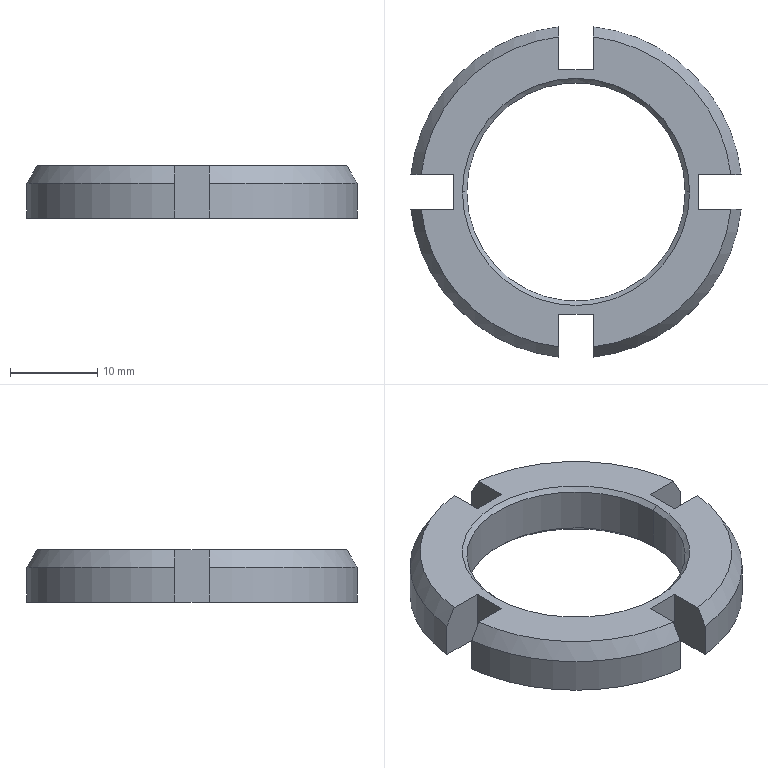Part | SolidWorks | features Chamfer 2, CirPattern 1, Extrusion 1, ICE 1 | 1 solid | 28 faces | box 37.789 x 37.789 x 6 mm | volume 3246 mm3 | plane 14 | cone 8 | cylinder 6 | commonest cylinder face diameters 38 x4 25 x2
STEP:
#1=CARTESIAN_POINT('',(12.5,0.,0.5));
#2=VERTEX_POINT('',#1);
#3=CARTESIAN_POINT('',(-12.5,0.,0.5));
#4=VERTEX_POINT('',#3);
#5=CARTESIAN_POINT('',(0.,0.,0.5));
#6=DIRECTION('',(0.,0.,-1.));
#7=DIRECTION('',(1.,0.,0.));
#8=AXIS2_PLACEMENT_3D('',#5,#6,#7);
#9=CIRCLE('',#8,12.5);
#10=EDGE_CURVE('',#2,#4,#9,.T.);
#11=ORIENTED_EDGE('',*,*,#10,.F.);
#12=CARTESIAN_POINT('',(13.,0.,0.));
#13=VERTEX_POINT('',#12);
#14=CARTESIAN_POINT('',(13.,0.,0.));
#15=DIRECTION('',(0.7071,0.,-0.7071));
#16=VECTOR('',#15,1000.);
#17=LINE('',#14,#16);
#18=EDGE_CURVE('',#2,#13,#17,.T.);
#19=ORIENTED_EDGE('',*,*,#18,.T.);
#20=CARTESIAN_POINT('',(-13.,0.,0.));
#21=VERTEX_POINT('',#20);
#22=CARTESIAN_POINT('',(0.,0.,0.));
#23=DIRECTION('',(0.,0.,1.));
#24=DIRECTION('',(1.,0.,0.));
#25=AXIS2_PLACEMENT_3D('',#22,#23,#24);
#26=CIRCLE('',#25,13.);
#27=EDGE_CURVE('',#21,#13,#26,.T.);
#28=ORIENTED_EDGE('',*,*,#27,.F.);
#29=CARTESIAN_POINT('',(-13.,0.,0.));
#30=DIRECTION('',(-0.7071,0.,-0.7071));
#31=VECTOR('',#30,1000.);
#32=LINE('',#29,#31);
#33=EDGE_CURVE('',#4,#21,#32,.T.);
#34=ORIENTED_EDGE('',*,*,#33,.F.);
#35=EDGE_LOOP('',(#11,#19,#28,#34));
#36=FACE_OUTER_BOUND('',#35,.T.);
#37=CARTESIAN_POINT('',(0.,0.,0.));
#38=DIRECTION('',(0.,0.,-1.));
#39=DIRECTION('',(-1.,0.,0.));
#40=AXIS2_PLACEMENT_3D('',#37,#38,#39);
#41=CONICAL_SURFACE('',#40,13.,0.7854);
#42=ADVANCED_FACE('',(#36),#41,.F.);
#43=CARTESIAN_POINT('',(-12.5,0.,5.5));
#44=VERTEX_POINT('',#43);
#45=CARTESIAN_POINT('',(12.5,0.,5.5));
#46=VERTEX_POINT('',#45);
#47=CARTESIAN_POINT('',(0.,0.,5.5));
#48=DIRECTION('',(0.,0.,1.));
#49=DIRECTION('',(1.,0.,0.));
#50=AXIS2_PLACEMENT_3D('',#47,#48,#49);
#51=CIRCLE('',#50,12.5);
#52=EDGE_CURVE('',#44,#46,#51,.T.);
#53=ORIENTED_EDGE('',*,*,#52,.F.);
#54=CARTESIAN_POINT('',(-13.,0.,6.));
#55=VERTEX_POINT('',#54);
#56=CARTESIAN_POINT('',(-12.5,0.,5.5));
#57=DIRECTION('',(-0.7071,0.,0.7071));
#58=VECTOR('',#57,1000.);
#59=LINE('',#56,#58);
#60=EDGE_CURVE('',#44,#55,#59,.T.);
#61=ORIENTED_EDGE('',*,*,#60,.T.);
#62=CARTESIAN_POINT('',(13.,0.,6.));
#63=VERTEX_POINT('',#62);
#64=CARTESIAN_POINT('',(0.,0.,6.));
#65=DIRECTION('',(0.,0.,-1.));
#66=DIRECTION('',(1.,0.,0.));
#67=AXIS2_PLACEMENT_3D('',#64,#65,#66);
#68=CIRCLE('',#67,13.);
#69=EDGE_CURVE('',#63,#55,#68,.T.);
#70=ORIENTED_EDGE('',*,*,#69,.F.);
#71=CARTESIAN_POINT('',(12.5,0.,5.5));
#72=DIRECTION('',(0.7071,0.,0.7071));
#73=VECTOR('',#72,1000.);
#74=LINE('',#71,#73);
#75=EDGE_CURVE('',#46,#63,#74,.T.);
#76=ORIENTED_EDGE('',*,*,#75,.F.);
#77=EDGE_LOOP('',(#53,#61,#70,#76));
#78=FACE_OUTER_BOUND('',#77,.T.);
#79=CARTESIAN_POINT('',(0.,0.,5.5));
#80=DIRECTION('',(0.,0.,1.));
#81=DIRECTION('',(1.,0.,0.));
#82=AXIS2_PLACEMENT_3D('',#79,#80,#81);
#83=CONICAL_SURFACE('',#82,12.5,0.7854);
#84=ADVANCED_FACE('',(#78),#83,.F.);
#85=ORIENTED_EDGE('',*,*,#52,.T.);
#86=CARTESIAN_POINT('',(12.5,0.,6.));
#87=DIRECTION('',(0.,0.,-1.));
#88=VECTOR('',#87,1000.);
#89=LINE('',#86,#88);
#90=EDGE_CURVE('',#46,#2,#89,.T.);
#91=ORIENTED_EDGE('',*,*,#90,.T.);
#92=ORIENTED_EDGE('',*,*,#10,.T.);
#93=CARTESIAN_POINT('',(-12.5,0.,6.));
#94=DIRECTION('',(0.,0.,-1.));
#95=VECTOR('',#94,1000.);
#96=LINE('',#93,#95);
#97=EDGE_CURVE('',#44,#4,#96,.T.);
#98=ORIENTED_EDGE('',*,*,#97,.F.);
#99=EDGE_LOOP('',(#85,#91,#92,#98));
#100=FACE_OUTER_BOUND('',#99,.T.);
#101=CARTESIAN_POINT('',(0.,0.,6.));
#102=DIRECTION('',(0.,0.,-1.));
#103=DIRECTION('',(-1.,0.,0.));
#104=AXIS2_PLACEMENT_3D('',#101,#102,#103);
#105=CYLINDRICAL_SURFACE('',#104,12.5);
#106=ADVANCED_FACE('',(#100),#105,.F.);
#107=ORIENTED_EDGE('',*,*,#69,.T.);
#108=CARTESIAN_POINT('',(0.,0.,6.));
#109=DIRECTION('',(0.,0.,-1.));
#110=DIRECTION('',(1.,0.,0.));
#111=AXIS2_PLACEMENT_3D('',#108,#109,#110);
#112=CIRCLE('',#111,13.);
#113=EDGE_CURVE('',#55,#63,#112,.T.);
#114=ORIENTED_EDGE('',*,*,#113,.T.);
#115=EDGE_LOOP('',(#107,#114));
#116=FACE_BOUND('',#115,.T.);
#117=CARTESIAN_POINT('',(2.,-17.733,6.));
#118=VERTEX_POINT('',#117);
#119=CARTESIAN_POINT('',(2.,-14.,6.));
#120=VERTEX_POINT('',#119);
#121=CARTESIAN_POINT('',(2.,-20.,6.));
#122=DIRECTION('',(0.,1.,0.));
#123=VECTOR('',#122,1000.);
#124=LINE('',#121,#123);
#125=EDGE_CURVE('',#118,#120,#124,.T.);
#126=ORIENTED_EDGE('',*,*,#125,.F.);
#127=CARTESIAN_POINT('',(17.733,-2.,6.));
#128=VERTEX_POINT('',#127);
#129=CARTESIAN_POINT('',(0.,0.,6.));
#130=DIRECTION('',(0.,0.,1.));
#131=DIRECTION('',(1.,0.,0.));
#132=AXIS2_PLACEMENT_3D('',#129,#130,#131);
#133=CIRCLE('',#132,17.845);
#134=EDGE_CURVE('',#118,#128,#133,.T.);
#135=ORIENTED_EDGE('',*,*,#134,.T.);
#136=CARTESIAN_POINT('',(14.,-2.,6.));
#137=VERTEX_POINT('',#136);
#138=CARTESIAN_POINT('',(20.,-2.,6.));
#139=DIRECTION('',(-1.,0.,0.));
#140=VECTOR('',#139,1000.);
#141=LINE('',#138,#140);
#142=EDGE_CURVE('',#128,#137,#141,.T.);
#143=ORIENTED_EDGE('',*,*,#142,.T.);
#144=CARTESIAN_POINT('',(14.,2.,6.));
#145=VERTEX_POINT('',#144);
#146=CARTESIAN_POINT('',(14.,-2.,6.));
#147=DIRECTION('',(0.,-1.,0.));
#148=VECTOR('',#147,1000.);
#149=LINE('',#146,#148);
#150=EDGE_CURVE('',#145,#137,#149,.T.);
#151=ORIENTED_EDGE('',*,*,#150,.F.);
#152=CARTESIAN_POINT('',(17.733,2.,6.));
#153=VERTEX_POINT('',#152);
#154=CARTESIAN_POINT('',(20.,2.,6.));
#155=DIRECTION('',(-1.,0.,0.));
#156=VECTOR('',#155,1000.);
#157=LINE('',#154,#156);
#158=EDGE_CURVE('',#153,#145,#157,.T.);
#159=ORIENTED_EDGE('',*,*,#158,.F.);
#160=CARTESIAN_POINT('',(2.,17.733,6.));
#161=VERTEX_POINT('',#160);
#162=CARTESIAN_POINT('',(0.,0.,6.));
#163=DIRECTION('',(0.,0.,1.));
#164=DIRECTION('',(1.,0.,0.));
#165=AXIS2_PLACEMENT_3D('',#162,#163,#164);
#166=CIRCLE('',#165,17.845);
#167=EDGE_CURVE('',#153,#161,#166,.T.);
#168=ORIENTED_EDGE('',*,*,#167,.T.);
#169=CARTESIAN_POINT('',(2.,14.,6.));
#170=VERTEX_POINT('',#169);
#171=CARTESIAN_POINT('',(2.,20.,6.));
#172=DIRECTION('',(0.,-1.,0.));
#173=VECTOR('',#172,1000.);
#174=LINE('',#171,#173);
#175=EDGE_CURVE('',#161,#170,#174,.T.);
#176=ORIENTED_EDGE('',*,*,#175,.T.);
#177=CARTESIAN_POINT('',(-2.,14.,6.));
#178=VERTEX_POINT('',#177);
#179=CARTESIAN_POINT('',(2.,14.,6.));
#180=DIRECTION('',(1.,0.,0.));
#181=VECTOR('',#180,1000.);
#182=LINE('',#179,#181);
#183=EDGE_CURVE('',#178,#170,#182,.T.);
#184=ORIENTED_EDGE('',*,*,#183,.F.);
#185=CARTESIAN_POINT('',(-2.,17.733,6.));
#186=VERTEX_POINT('',#185);
#187=CARTESIAN_POINT('',(-2.,20.,6.));
#188=DIRECTION('',(0.,-1.,0.));
#189=VECTOR('',#188,1000.);
#190=LINE('',#187,#189);
#191=EDGE_CURVE('',#186,#178,#190,.T.);
#192=ORIENTED_EDGE('',*,*,#191,.F.);
#193=CARTESIAN_POINT('',(-17.733,2.,6.));
#194=VERTEX_POINT('',#193);
#195=CARTESIAN_POINT('',(0.,0.,6.));
#196=DIRECTION('',(0.,0.,1.));
#197=DIRECTION('',(1.,0.,0.));
#198=AXIS2_PLACEMENT_3D('',#195,#196,#197);
#199=CIRCLE('',#198,17.845);
#200=EDGE_CURVE('',#186,#194,#199,.T.);
#201=ORIENTED_EDGE('',*,*,#200,.T.);
#202=CARTESIAN_POINT('',(-14.,2.,6.));
#203=VERTEX_POINT('',#202);
#204=CARTESIAN_POINT('',(-20.,2.,6.));
#205=DIRECTION('',(1.,0.,0.));
#206=VECTOR('',#205,1000.);
#207=LINE('',#204,#206);
#208=EDGE_CURVE('',#194,#203,#207,.T.);
#209=ORIENTED_EDGE('',*,*,#208,.T.);
#210=CARTESIAN_POINT('',(-14.,-2.,6.));
#211=VERTEX_POINT('',#210);
#212=CARTESIAN_POINT('',(-14.,2.,6.));
#213=DIRECTION('',(0.,1.,0.));
#214=VECTOR('',#213,1000.);
#215=LINE('',#212,#214);
#216=EDGE_CURVE('',#211,#203,#215,.T.);
#217=ORIENTED_EDGE('',*,*,#216,.F.);
#218=CARTESIAN_POINT('',(-17.733,-2.,6.));
#219=VERTEX_POINT('',#218);
#220=CARTESIAN_POINT('',(-20.,-2.,6.));
#221=DIRECTION('',(1.,0.,0.));
#222=VECTOR('',#221,1000.);
#223=LINE('',#220,#222);
#224=EDGE_CURVE('',#219,#211,#223,.T.);
#225=ORIENTED_EDGE('',*,*,#224,.F.);
#226=CARTESIAN_POINT('',(-2.,-17.733,6.));
#227=VERTEX_POINT('',#226);
#228=CARTESIAN_POINT('',(0.,0.,6.));
#229=DIRECTION('',(0.,0.,1.));
#230=DIRECTION('',(1.,0.,0.));
#231=AXIS2_PLACEMENT_3D('',#228,#229,#230);
#232=CIRCLE('',#231,17.845);
#233=EDGE_CURVE('',#219,#227,#232,.T.);
#234=ORIENTED_EDGE('',*,*,#233,.T.);
#235=CARTESIAN_POINT('',(-2.,-14.,6.));
#236=VERTEX_POINT('',#235);
#237=CARTESIAN_POINT('',(-2.,-20.,6.));
#238=DIRECTION('',(0.,1.,0.));
#239=VECTOR('',#238,1000.);
#240=LINE('',#237,#239);
#241=EDGE_CURVE('',#227,#236,#240,.T.);
#242=ORIENTED_EDGE('',*,*,#241,.T.);
#243=CARTESIAN_POINT('',(-2.,-14.,6.));
#244=DIRECTION('',(-1.,0.,0.));
#245=VECTOR('',#244,1000.);
#246=LINE('',#243,#245);
#247=EDGE_CURVE('',#120,#236,#246,.T.);
#248=ORIENTED_EDGE('',*,*,#247,.F.);
#249=EDGE_LOOP('',(#126,#135,#143,#151,#159,#168,#176,#184,#192,#201,#209,#217,#225,#234,#242,#248));
#250=FACE_OUTER_BOUND('',#249,.T.);
#251=CARTESIAN_POINT('',(0.,0.,6.));
#252=DIRECTION('',(0.,0.,1.));
#253=DIRECTION('',(1.,0.,0.));
#254=AXIS2_PLACEMENT_3D('',#251,#252,#253);
#255=PLANE('',#254);
#256=ADVANCED_FACE('',(#116,#250),#255,.T.);
#257=ORIENTED_EDGE('',*,*,#27,.T.);
#258=CARTESIAN_POINT('',(0.,0.,0.));
#259=DIRECTION('',(0.,0.,1.));
#260=DIRECTION('',(1.,0.,0.));
#261=AXIS2_PLACEMENT_3D('',#258,#259,#260);
#262=CIRCLE('',#261,13.);
#263=EDGE_CURVE('',#13,#21,#262,.T.);
#264=ORIENTED_EDGE('',*,*,#263,.T.);
#265=EDGE_LOOP('',(#257,#264));
#266=FACE_BOUND('',#265,.T.);
#267=CARTESIAN_POINT('',(-2.,18.894,0.));
#268=VERTEX_POINT('',#267);
#269=CARTESIAN_POINT('',(-2.,14.,0.));
#270=VERTEX_POINT('',#269);
#271=CARTESIAN_POINT('',(-2.,20.,0.));
#272=DIRECTION('',(0.,-1.,0.));
#273=VECTOR('',#272,1000.);
#274=LINE('',#271,#273);
#275=EDGE_CURVE('',#268,#270,#274,.T.);
#276=ORIENTED_EDGE('',*,*,#275,.T.);
#277=CARTESIAN_POINT('',(2.,14.,0.));
#278=VERTEX_POINT('',#277);
#279=CARTESIAN_POINT('',(2.,14.,0.));
#280=DIRECTION('',(-1.,0.,0.));
#281=VECTOR('',#280,1000.);
#282=LINE('',#279,#281);
#283=EDGE_CURVE('',#278,#270,#282,.T.);
#284=ORIENTED_EDGE('',*,*,#283,.F.);
#285=CARTESIAN_POINT('',(2.,18.894,0.));
#286=VERTEX_POINT('',#285);
#287=CARTESIAN_POINT('',(2.,20.,0.));
#288=DIRECTION('',(0.,-1.,0.));
#289=VECTOR('',#288,1000.);
#290=LINE('',#287,#289);
#291=EDGE_CURVE('',#286,#278,#290,.T.);
#292=ORIENTED_EDGE('',*,*,#291,.F.);
#293=CARTESIAN_POINT('',(18.894,2.,0.));
#294=VERTEX_POINT('',#293);
#295=CARTESIAN_POINT('',(0.,0.,0.));
#296=DIRECTION('',(0.,0.,1.));
#297=DIRECTION('',(1.,0.,0.));
#298=AXIS2_PLACEMENT_3D('',#295,#296,#297);
#299=CIRCLE('',#298,19.);
#300=EDGE_CURVE('',#294,#286,#299,.T.);
#301=ORIENTED_EDGE('',*,*,#300,.F.);
#302=CARTESIAN_POINT('',(14.,2.,0.));
#303=VERTEX_POINT('',#302);
#304=CARTESIAN_POINT('',(20.,2.,0.));
#305=DIRECTION('',(-1.,0.,0.));
#306=VECTOR('',#305,1000.);
#307=LINE('',#304,#306);
#308=EDGE_CURVE('',#294,#303,#307,.T.);
#309=ORIENTED_EDGE('',*,*,#308,.T.);
#310=CARTESIAN_POINT('',(14.,-2.,0.));
#311=VERTEX_POINT('',#310);
#312=CARTESIAN_POINT('',(14.,-2.,0.));
#313=DIRECTION('',(0.,1.,0.));
#314=VECTOR('',#313,1000.);
#315=LINE('',#312,#314);
#316=EDGE_CURVE('',#311,#303,#315,.T.);
#317=ORIENTED_EDGE('',*,*,#316,.F.);
#318=CARTESIAN_POINT('',(18.894,-2.,0.));
#319=VERTEX_POINT('',#318);
#320=CARTESIAN_POINT('',(20.,-2.,0.));
#321=DIRECTION('',(-1.,0.,0.));
#322=VECTOR('',#321,1000.);
#323=LINE('',#320,#322);
#324=EDGE_CURVE('',#319,#311,#323,.T.);
#325=ORIENTED_EDGE('',*,*,#324,.F.);
#326=CARTESIAN_POINT('',(2.,-18.894,0.));
#327=VERTEX_POINT('',#326);
#328=CARTESIAN_POINT('',(0.,0.,0.));
#329=DIRECTION('',(0.,0.,1.));
#330=DIRECTION('',(1.,0.,0.));
#331=AXIS2_PLACEMENT_3D('',#328,#329,#330);
#332=CIRCLE('',#331,19.);
#333=EDGE_CURVE('',#327,#319,#332,.T.);
#334=ORIENTED_EDGE('',*,*,#333,.F.);
#335=CARTESIAN_POINT('',(2.,-14.,0.));
#336=VERTEX_POINT('',#335);
#337=CARTESIAN_POINT('',(2.,-20.,0.));
#338=DIRECTION('',(0.,1.,0.));
#339=VECTOR('',#338,1000.);
#340=LINE('',#337,#339);
#341=EDGE_CURVE('',#327,#336,#340,.T.);
#342=ORIENTED_EDGE('',*,*,#341,.T.);
#343=CARTESIAN_POINT('',(-2.,-14.,0.));
#344=VERTEX_POINT('',#343);
#345=CARTESIAN_POINT('',(-2.,-14.,0.));
#346=DIRECTION('',(1.,0.,0.));
#347=VECTOR('',#346,1000.);
#348=LINE('',#345,#347);
#349=EDGE_CURVE('',#344,#336,#348,.T.);
#350=ORIENTED_EDGE('',*,*,#349,.F.);
#351=CARTESIAN_POINT('',(-2.,-18.894,0.));
#352=VERTEX_POINT('',#351);
#353=CARTESIAN_POINT('',(-2.,-20.,0.));
#354=DIRECTION('',(0.,1.,0.));
#355=VECTOR('',#354,1000.);
#356=LINE('',#353,#355);
#357=EDGE_CURVE('',#352,#344,#356,.T.);
#358=ORIENTED_EDGE('',*,*,#357,.F.);
#359=CARTESIAN_POINT('',(-18.894,-2.,0.));
#360=VERTEX_POINT('',#359);
#361=CARTESIAN_POINT('',(0.,0.,0.));
#362=DIRECTION('',(0.,0.,1.));
#363=DIRECTION('',(1.,0.,0.));
#364=AXIS2_PLACEMENT_3D('',#361,#362,#363);
#365=CIRCLE('',#364,19.);
#366=EDGE_CURVE('',#360,#352,#365,.T.);
#367=ORIENTED_EDGE('',*,*,#366,.F.);
#368=CARTESIAN_POINT('',(-14.,-2.,0.));
#369=VERTEX_POINT('',#368);
#370=CARTESIAN_POINT('',(-20.,-2.,0.));
#371=DIRECTION('',(1.,0.,0.));
#372=VECTOR('',#371,1000.);
#373=LINE('',#370,#372);
#374=EDGE_CURVE('',#360,#369,#373,.T.);
#375=ORIENTED_EDGE('',*,*,#374,.T.);
#376=CARTESIAN_POINT('',(-14.,2.,0.));
#377=VERTEX_POINT('',#376);
#378=CARTESIAN_POINT('',(-14.,2.,0.));
#379=DIRECTION('',(0.,-1.,0.));
#380=VECTOR('',#379,1000.);
#381=LINE('',#378,#380);
#382=EDGE_CURVE('',#377,#369,#381,.T.);
#383=ORIENTED_EDGE('',*,*,#382,.F.);
#384=CARTESIAN_POINT('',(-18.894,2.,0.));
#385=VERTEX_POINT('',#384);
#386=CARTESIAN_POINT('',(-20.,2.,0.));
#387=DIRECTION('',(1.,0.,0.));
#388=VECTOR('',#387,1000.);
#389=LINE('',#386,#388);
#390=EDGE_CURVE('',#385,#377,#389,.T.);
#391=ORIENTED_EDGE('',*,*,#390,.F.);
#392=CARTESIAN_POINT('',(0.,0.,0.));
#393=DIRECTION('',(0.,0.,1.));
#394=DIRECTION('',(1.,0.,0.));
#395=AXIS2_PLACEMENT_3D('',#392,#393,#394);
#396=CIRCLE('',#395,19.);
#397=EDGE_CURVE('',#268,#385,#396,.T.);
#398=ORIENTED_EDGE('',*,*,#397,.F.);
#399=EDGE_LOOP('',(#276,#284,#292,#301,#309,#317,#325,#334,#342,#350,#358,#367,#375,#383,#391,#398));
#400=FACE_OUTER_BOUND('',#399,.T.);
#401=CARTESIAN_POINT('',(0.,0.,0.));
#402=DIRECTION('',(0.,0.,1.));
#403=DIRECTION('',(1.,0.,0.));
#404=AXIS2_PLACEMENT_3D('',#401,#402,#403);
#405=PLANE('',#404);
#406=ADVANCED_FACE('',(#266,#400),#405,.F.);
#407=CARTESIAN_POINT('',(-18.894,2.,4.));
#408=VERTEX_POINT('',#407);
#409=CARTESIAN_POINT('',(-18.894,2.,6.));
#410=DIRECTION('',(0.,0.,-1.));
#411=VECTOR('',#410,1000.);
#412=LINE('',#409,#411);
#413=EDGE_CURVE('',#408,#385,#412,.T.);
#414=ORIENTED_EDGE('',*,*,#413,.F.);
#415=CARTESIAN_POINT('',(-2.,18.894,4.));
#416=VERTEX_POINT('',#415);
#417=CARTESIAN_POINT('',(0.,0.,4.));
#418=DIRECTION('',(0.,0.,-1.));
#419=DIRECTION('',(1.,0.,0.));
#420=AXIS2_PLACEMENT_3D('',#417,#418,#419);
#421=CIRCLE('',#420,19.);
#422=EDGE_CURVE('',#408,#416,#421,.T.);
#423=ORIENTED_EDGE('',*,*,#422,.T.);
#424=CARTESIAN_POINT('',(-2.,18.894,6.));
#425=DIRECTION('',(0.,0.,1.));
#426=VECTOR('',#425,1000.);
#427=LINE('',#424,#426);
#428=EDGE_CURVE('',#268,#416,#427,.T.);
#429=ORIENTED_EDGE('',*,*,#428,.F.);
#430=ORIENTED_EDGE('',*,*,#397,.T.);
#431=EDGE_LOOP('',(#414,#423,#429,#430));
#432=FACE_OUTER_BOUND('',#431,.T.);
#433=CARTESIAN_POINT('',(0.,0.,6.));
#434=DIRECTION('',(0.,0.,-1.));
#435=DIRECTION('',(-1.,0.,0.));
#436=AXIS2_PLACEMENT_3D('',#433,#434,#435);
#437=CYLINDRICAL_SURFACE('',#436,19.);
#438=ADVANCED_FACE('',(#432),#437,.T.);
#439=CARTESIAN_POINT('',(2.,18.894,4.));
#440=VERTEX_POINT('',#439);
#441=CARTESIAN_POINT('',(2.,18.894,6.));
#442=DIRECTION('',(0.,0.,-1.));
#443=VECTOR('',#442,1000.);
#444=LINE('',#441,#443);
#445=EDGE_CURVE('',#440,#286,#444,.T.);
#446=ORIENTED_EDGE('',*,*,#445,.F.);
#447=CARTESIAN_POINT('',(18.894,2.,4.));
#448=VERTEX_POINT('',#447);
#449=CARTESIAN_POINT('',(0.,0.,4.));
#450=DIRECTION('',(0.,0.,-1.));
#451=DIRECTION('',(1.,0.,0.));
#452=AXIS2_PLACEMENT_3D('',#449,#450,#451);
#453=CIRCLE('',#452,19.);
#454=EDGE_CURVE('',#440,#448,#453,.T.);
#455=ORIENTED_EDGE('',*,*,#454,.T.);
#456=CARTESIAN_POINT('',(18.894,2.,6.));
#457=DIRECTION('',(0.,0.,1.));
#458=VECTOR('',#457,1000.);
#459=LINE('',#456,#458);
#460=EDGE_CURVE('',#294,#448,#459,.T.);
#461=ORIENTED_EDGE('',*,*,#460,.F.);
#462=ORIENTED_EDGE('',*,*,#300,.T.);
#463=EDGE_LOOP('',(#446,#455,#461,#462));
#464=FACE_OUTER_BOUND('',#463,.T.);
#465=CARTESIAN_POINT('',(0.,0.,6.));
#466=DIRECTION('',(0.,0.,-1.));
#467=DIRECTION('',(-1.,0.,0.));
#468=AXIS2_PLACEMENT_3D('',#465,#466,#467);
#469=CYLINDRICAL_SURFACE('',#468,19.);
#470=ADVANCED_FACE('',(#464),#469,.T.);
#471=CARTESIAN_POINT('',(-2.,-18.894,4.));
#472=VERTEX_POINT('',#471);
#473=CARTESIAN_POINT('',(-2.,-18.894,6.));
#474=DIRECTION('',(0.,0.,-1.));
#475=VECTOR('',#474,1000.);
#476=LINE('',#473,#475);
#477=EDGE_CURVE('',#472,#352,#476,.T.);
#478=ORIENTED_EDGE('',*,*,#477,.F.);
#479=CARTESIAN_POINT('',(-18.894,-2.,4.));
#480=VERTEX_POINT('',#479);
#481=CARTESIAN_POINT('',(0.,0.,4.));
#482=DIRECTION('',(0.,0.,-1.));
#483=DIRECTION('',(1.,0.,0.));
#484=AXIS2_PLACEMENT_3D('',#481,#482,#483);
#485=CIRCLE('',#484,19.);
#486=EDGE_CURVE('',#472,#480,#485,.T.);
#487=ORIENTED_EDGE('',*,*,#486,.T.);
#488=CARTESIAN_POINT('',(-18.894,-2.,6.));
#489=DIRECTION('',(0.,0.,1.));
#490=VECTOR('',#489,1000.);
#491=LINE('',#488,#490);
#492=EDGE_CURVE('',#360,#480,#491,.T.);
#493=ORIENTED_EDGE('',*,*,#492,.F.);
#494=ORIENTED_EDGE('',*,*,#366,.T.);
#495=EDGE_LOOP('',(#478,#487,#493,#494));
#496=FACE_OUTER_BOUND('',#495,.T.);
#497=CARTESIAN_POINT('',(0.,0.,6.));
#498=DIRECTION('',(0.,0.,-1.));
#499=DIRECTION('',(-1.,0.,0.));
#500=AXIS2_PLACEMENT_3D('',#497,#498,#499);
#501=CYLINDRICAL_SURFACE('',#500,19.);
#502=ADVANCED_FACE('',(#496),#501,.T.);
#503=CARTESIAN_POINT('',(18.894,-2.,4.));
#504=VERTEX_POINT('',#503);
#505=CARTESIAN_POINT('',(18.894,-2.,6.));
#506=DIRECTION('',(0.,0.,-1.));
#507=VECTOR('',#506,1000.);
#508=LINE('',#505,#507);
#509=EDGE_CURVE('',#504,#319,#508,.T.);
#510=ORIENTED_EDGE('',*,*,#509,.F.);
#511=CARTESIAN_POINT('',(2.,-18.894,4.));
#512=VERTEX_POINT('',#511);
#513=CARTESIAN_POINT('',(0.,0.,4.));
#514=DIRECTION('',(0.,0.,-1.));
#515=DIRECTION('',(1.,0.,0.));
#516=AXIS2_PLACEMENT_3D('',#513,#514,#515);
#517=CIRCLE('',#516,19.);
#518=EDGE_CURVE('',#504,#512,#517,.T.);
#519=ORIENTED_EDGE('',*,*,#518,.T.);
#520=CARTESIAN_POINT('',(2.,-18.894,6.));
#521=DIRECTION('',(0.,0.,1.));
#522=VECTOR('',#521,1000.);
#523=LINE('',#520,#522);
#524=EDGE_CURVE('',#327,#512,#523,.T.);
#525=ORIENTED_EDGE('',*,*,#524,.F.);
#526=ORIENTED_EDGE('',*,*,#333,.T.);
#527=EDGE_LOOP('',(#510,#519,#525,#526));
#528=FACE_OUTER_BOUND('',#527,.T.);
#529=CARTESIAN_POINT('',(0.,0.,6.));
#530=DIRECTION('',(0.,0.,-1.));
#531=DIRECTION('',(-1.,0.,0.));
#532=AXIS2_PLACEMENT_3D('',#529,#530,#531);
#533=CYLINDRICAL_SURFACE('',#532,19.);
#534=ADVANCED_FACE('',(#528),#533,.T.);
#535=ORIENTED_EDGE('',*,*,#90,.F.);
#536=CARTESIAN_POINT('',(0.,0.,5.5));
#537=DIRECTION('',(0.,0.,1.));
#538=DIRECTION('',(1.,0.,0.));
#539=AXIS2_PLACEMENT_3D('',#536,#537,#538);
#540=CIRCLE('',#539,12.5);
#541=EDGE_CURVE('',#46,#44,#540,.T.);
#542=ORIENTED_EDGE('',*,*,#541,.T.);
#543=ORIENTED_EDGE('',*,*,#97,.T.);
#544=CARTESIAN_POINT('',(0.,0.,0.5));
#545=DIRECTION('',(0.,0.,-1.));
#546=DIRECTION('',(1.,0.,0.));
#547=AXIS2_PLACEMENT_3D('',#544,#545,#546);
#548=CIRCLE('',#547,12.5);
#549=EDGE_CURVE('',#4,#2,#548,.T.);
#550=ORIENTED_EDGE('',*,*,#549,.T.);
#551=EDGE_LOOP('',(#535,#542,#543,#550));
#552=FACE_OUTER_BOUND('',#551,.T.);
#553=CARTESIAN_POINT('',(0.,0.,6.));
#554=DIRECTION('',(0.,0.,-1.));
#555=DIRECTION('',(-1.,0.,0.));
#556=AXIS2_PLACEMENT_3D('',#553,#554,#555);
#557=CYLINDRICAL_SURFACE('',#556,12.5);
#558=ADVANCED_FACE('',(#552),#557,.F.);
#559=ORIENTED_EDGE('',*,*,#460,.T.);
#560=CARTESIAN_POINT('',(18.894,2.,4.));
#561=CARTESIAN_POINT('',(18.507,2.,4.667));
#562=CARTESIAN_POINT('',(18.12,2.,5.333));
#563=CARTESIAN_POINT('',(17.733,2.,6.));
#564=B_SPLINE_CURVE_WITH_KNOTS('',3,(#560,#561,#562,#563),.UNSPECIFIED.,.F.,.F.,(4,4),(0.,0.002313),.UNSPECIFIED.);
#565=EDGE_CURVE('',#448,#153,#564,.T.);
#566=ORIENTED_EDGE('',*,*,#565,.T.);
#567=ORIENTED_EDGE('',*,*,#158,.T.);
#568=CARTESIAN_POINT('',(14.,2.,0.));
#569=DIRECTION('',(0.,0.,1.));
#570=VECTOR('',#569,1000.);
#571=LINE('',#568,#570);
#572=EDGE_CURVE('',#303,#145,#571,.T.);
#573=ORIENTED_EDGE('',*,*,#572,.F.);
#574=ORIENTED_EDGE('',*,*,#308,.F.);
#575=EDGE_LOOP('',(#559,#566,#567,#573,#574));
#576=FACE_OUTER_BOUND('',#575,.T.);
#577=CARTESIAN_POINT('',(20.,2.,0.));
#578=DIRECTION('',(0.,-1.,0.));
#579=DIRECTION('',(0.,0.,-1.));
#580=AXIS2_PLACEMENT_3D('',#577,#578,#579);
#581=PLANE('',#580);
#582=ADVANCED_FACE('',(#576),#581,.T.);
#583=ORIENTED_EDGE('',*,*,#142,.F.);
#584=CARTESIAN_POINT('',(17.733,-2.,6.));
#585=CARTESIAN_POINT('',(18.12,-2.,5.333));
#586=CARTESIAN_POINT('',(18.507,-2.,4.667));
#587=CARTESIAN_POINT('',(18.894,-2.,4.));
#588=B_SPLINE_CURVE_WITH_KNOTS('',3,(#584,#585,#586,#587),.UNSPECIFIED.,.F.,.F.,(4,4),(0.,0.002313),.UNSPECIFIED.);
#589=EDGE_CURVE('',#128,#504,#588,.T.);
#590=ORIENTED_EDGE('',*,*,#589,.T.);
#591=ORIENTED_EDGE('',*,*,#509,.T.);
#592=ORIENTED_EDGE('',*,*,#324,.T.);
#593=CARTESIAN_POINT('',(14.,-2.,0.));
#594=DIRECTION('',(0.,0.,-1.));
#595=VECTOR('',#594,1000.);
#596=LINE('',#593,#595);
#597=EDGE_CURVE('',#137,#311,#596,.T.);
#598=ORIENTED_EDGE('',*,*,#597,.F.);
#599=EDGE_LOOP('',(#583,#590,#591,#592,#598));
#600=FACE_OUTER_BOUND('',#599,.T.);
#601=CARTESIAN_POINT('',(20.,-2.,0.));
#602=DIRECTION('',(0.,1.,0.));
#603=DIRECTION('',(0.,0.,1.));
#604=AXIS2_PLACEMENT_3D('',#601,#602,#603);
#605=PLANE('',#604);
#606=ADVANCED_FACE('',(#600),#605,.T.);
#607=ORIENTED_EDGE('',*,*,#316,.T.);
#608=ORIENTED_EDGE('',*,*,#572,.T.);
#609=ORIENTED_EDGE('',*,*,#150,.T.);
#610=ORIENTED_EDGE('',*,*,#597,.T.);
#611=EDGE_LOOP('',(#607,#608,#609,#610));
#612=FACE_OUTER_BOUND('',#611,.T.);
#613=CARTESIAN_POINT('',(14.,2.,0.));
#614=DIRECTION('',(1.,0.,0.));
#615=DIRECTION('',(0.,0.,-1.));
#616=AXIS2_PLACEMENT_3D('',#613,#614,#615);
#617=PLANE('',#616);
#618=ADVANCED_FACE('',(#612),#617,.T.);
#619=ORIENTED_EDGE('',*,*,#349,.T.);
#620=CARTESIAN_POINT('',(2.,-14.,0.));
#621=DIRECTION('',(0.,0.,1.));
#622=VECTOR('',#621,1000.);
#623=LINE('',#620,#622);
#624=EDGE_CURVE('',#336,#120,#623,.T.);
#625=ORIENTED_EDGE('',*,*,#624,.T.);
#626=ORIENTED_EDGE('',*,*,#247,.T.);
#627=CARTESIAN_POINT('',(-2.,-14.,0.));
#628=DIRECTION('',(0.,0.,-1.));
#629=VECTOR('',#628,1000.);
#630=LINE('',#627,#629);
#631=EDGE_CURVE('',#236,#344,#630,.T.);
#632=ORIENTED_EDGE('',*,*,#631,.T.);
#633=EDGE_LOOP('',(#619,#625,#626,#632));
#634=FACE_OUTER_BOUND('',#633,.T.);
#635=CARTESIAN_POINT('',(2.,-14.,0.));
#636=DIRECTION('',(0.,-1.,0.));
#637=DIRECTION('',(0.,0.,-1.));
#638=AXIS2_PLACEMENT_3D('',#635,#636,#637);
#639=PLANE('',#638);
#640=ADVANCED_FACE('',(#634),#639,.T.);
#641=ORIENTED_EDGE('',*,*,#241,.F.);
#642=CARTESIAN_POINT('',(-2.,-17.733,6.));
#643=CARTESIAN_POINT('',(-2.,-18.12,5.333));
#644=CARTESIAN_POINT('',(-2.,-18.507,4.667));
#645=CARTESIAN_POINT('',(-2.,-18.894,4.));
#646=B_SPLINE_CURVE_WITH_KNOTS('',3,(#642,#643,#644,#645),.UNSPECIFIED.,.F.,.F.,(4,4),(0.,0.002313),.UNSPECIFIED.);
#647=EDGE_CURVE('',#227,#472,#646,.T.);
#648=ORIENTED_EDGE('',*,*,#647,.T.);
#649=ORIENTED_EDGE('',*,*,#477,.T.);
#650=ORIENTED_EDGE('',*,*,#357,.T.);
#651=ORIENTED_EDGE('',*,*,#631,.F.);
#652=EDGE_LOOP('',(#641,#648,#649,#650,#651));
#653=FACE_OUTER_BOUND('',#652,.T.);
#654=CARTESIAN_POINT('',(-2.,-20.,0.));
#655=DIRECTION('',(1.,0.,0.));
#656=DIRECTION('',(0.,0.,1.));
#657=AXIS2_PLACEMENT_3D('',#654,#655,#656);
#658=PLANE('',#657);
#659=ADVANCED_FACE('',(#653),#658,.T.);
#660=ORIENTED_EDGE('',*,*,#524,.T.);
#661=CARTESIAN_POINT('',(2.,-18.894,4.));
#662=CARTESIAN_POINT('',(2.,-18.507,4.667));
#663=CARTESIAN_POINT('',(2.,-18.12,5.333));
#664=CARTESIAN_POINT('',(2.,-17.733,6.));
#665=B_SPLINE_CURVE_WITH_KNOTS('',3,(#661,#662,#663,#664),.UNSPECIFIED.,.F.,.F.,(4,4),(0.,0.002313),.UNSPECIFIED.);
#666=EDGE_CURVE('',#512,#118,#665,.T.);
#667=ORIENTED_EDGE('',*,*,#666,.T.);
#668=ORIENTED_EDGE('',*,*,#125,.T.);
#669=ORIENTED_EDGE('',*,*,#624,.F.);
#670=ORIENTED_EDGE('',*,*,#341,.F.);
#671=EDGE_LOOP('',(#660,#667,#668,#669,#670));
#672=FACE_OUTER_BOUND('',#671,.T.);
#673=CARTESIAN_POINT('',(2.,-20.,0.));
#674=DIRECTION('',(-1.,0.,0.));
#675=DIRECTION('',(0.,0.,-1.));
#676=AXIS2_PLACEMENT_3D('',#673,#674,#675);
#677=PLANE('',#676);
#678=ADVANCED_FACE('',(#672),#677,.T.);
#679=ORIENTED_EDGE('',*,*,#382,.T.);
#680=CARTESIAN_POINT('',(-14.,-2.,0.));
#681=DIRECTION('',(0.,0.,1.));
#682=VECTOR('',#681,1000.);
#683=LINE('',#680,#682);
#684=EDGE_CURVE('',#369,#211,#683,.T.);
#685=ORIENTED_EDGE('',*,*,#684,.T.);
#686=ORIENTED_EDGE('',*,*,#216,.T.);
#687=CARTESIAN_POINT('',(-14.,2.,0.));
#688=DIRECTION('',(0.,0.,-1.));
#689=VECTOR('',#688,1000.);
#690=LINE('',#687,#689);
#691=EDGE_CURVE('',#203,#377,#690,.T.);
#692=ORIENTED_EDGE('',*,*,#691,.T.);
#693=EDGE_LOOP('',(#679,#685,#686,#692));
#694=FACE_OUTER_BOUND('',#693,.T.);
#695=CARTESIAN_POINT('',(-14.,-2.,0.));
#696=DIRECTION('',(-1.,0.,0.));
#697=DIRECTION('',(0.,0.,-1.));
#698=AXIS2_PLACEMENT_3D('',#695,#696,#697);
#699=PLANE('',#698);
#700=ADVANCED_FACE('',(#694),#699,.T.);
#701=ORIENTED_EDGE('',*,*,#208,.F.);
#702=CARTESIAN_POINT('',(-17.733,2.,6.));
#703=CARTESIAN_POINT('',(-18.12,2.,5.333));
#704=CARTESIAN_POINT('',(-18.507,2.,4.667));
#705=CARTESIAN_POINT('',(-18.894,2.,4.));
#706=B_SPLINE_CURVE_WITH_KNOTS('',3,(#702,#703,#704,#705),.UNSPECIFIED.,.F.,.F.,(4,4),(0.,0.002313),.UNSPECIFIED.);
#707=EDGE_CURVE('',#194,#408,#706,.T.);
#708=ORIENTED_EDGE('',*,*,#707,.T.);
#709=ORIENTED_EDGE('',*,*,#413,.T.);
#710=ORIENTED_EDGE('',*,*,#390,.T.);
#711=ORIENTED_EDGE('',*,*,#691,.F.);
#712=EDGE_LOOP('',(#701,#708,#709,#710,#711));
#713=FACE_OUTER_BOUND('',#712,.T.);
#714=CARTESIAN_POINT('',(-20.,2.,0.));
#715=DIRECTION('',(0.,-1.,0.));
#716=DIRECTION('',(0.,0.,1.));
#717=AXIS2_PLACEMENT_3D('',#714,#715,#716);
#718=PLANE('',#717);
#719=ADVANCED_FACE('',(#713),#718,.T.);
#720=ORIENTED_EDGE('',*,*,#492,.T.);
#721=CARTESIAN_POINT('',(-18.894,-2.,4.));
#722=CARTESIAN_POINT('',(-18.507,-2.,4.667));
#723=CARTESIAN_POINT('',(-18.12,-2.,5.333));
#724=CARTESIAN_POINT('',(-17.733,-2.,6.));
#725=B_SPLINE_CURVE_WITH_KNOTS('',3,(#721,#722,#723,#724),.UNSPECIFIED.,.F.,.F.,(4,4),(0.,0.002313),.UNSPECIFIED.);
#726=EDGE_CURVE('',#480,#219,#725,.T.);
#727=ORIENTED_EDGE('',*,*,#726,.T.);
#728=ORIENTED_EDGE('',*,*,#224,.T.);
#729=ORIENTED_EDGE('',*,*,#684,.F.);
#730=ORIENTED_EDGE('',*,*,#374,.F.);
#731=EDGE_LOOP('',(#720,#727,#728,#729,#730));
#732=FACE_OUTER_BOUND('',#731,.T.);
#733=CARTESIAN_POINT('',(-20.,-2.,0.));
#734=DIRECTION('',(0.,1.,0.));
#735=DIRECTION('',(0.,0.,-1.));
#736=AXIS2_PLACEMENT_3D('',#733,#734,#735);
#737=PLANE('',#736);
#738=ADVANCED_FACE('',(#732),#737,.T.);
#739=ORIENTED_EDGE('',*,*,#283,.T.);
#740=CARTESIAN_POINT('',(-2.,14.,0.));
#741=DIRECTION('',(0.,0.,1.));
#742=VECTOR('',#741,1000.);
#743=LINE('',#740,#742);
#744=EDGE_CURVE('',#270,#178,#743,.T.);
#745=ORIENTED_EDGE('',*,*,#744,.T.);
#746=ORIENTED_EDGE('',*,*,#183,.T.);
#747=CARTESIAN_POINT('',(2.,14.,0.));
#748=DIRECTION('',(0.,0.,-1.));
#749=VECTOR('',#748,1000.);
#750=LINE('',#747,#749);
#751=EDGE_CURVE('',#170,#278,#750,.T.);
#752=ORIENTED_EDGE('',*,*,#751,.T.);
#753=EDGE_LOOP('',(#739,#745,#746,#752));
#754=FACE_OUTER_BOUND('',#753,.T.);
#755=CARTESIAN_POINT('',(-2.,14.,0.));
#756=DIRECTION('',(0.,1.,0.));
#757=DIRECTION('',(0.,0.,-1.));
#758=AXIS2_PLACEMENT_3D('',#755,#756,#757);
#759=PLANE('',#758);
#760=ADVANCED_FACE('',(#754),#759,.T.);
#761=ORIENTED_EDGE('',*,*,#175,.F.);
#762=CARTESIAN_POINT('',(2.,17.733,6.));
#763=CARTESIAN_POINT('',(2.,18.12,5.333));
#764=CARTESIAN_POINT('',(2.,18.507,4.667));
#765=CARTESIAN_POINT('',(2.,18.894,4.));
#766=B_SPLINE_CURVE_WITH_KNOTS('',3,(#762,#763,#764,#765),.UNSPECIFIED.,.F.,.F.,(4,4),(0.,0.002313),.UNSPECIFIED.);
#767=EDGE_CURVE('',#161,#440,#766,.T.);
#768=ORIENTED_EDGE('',*,*,#767,.T.);
#769=ORIENTED_EDGE('',*,*,#445,.T.);
#770=ORIENTED_EDGE('',*,*,#291,.T.);
#771=ORIENTED_EDGE('',*,*,#751,.F.);
#772=EDGE_LOOP('',(#761,#768,#769,#770,#771));
#773=FACE_OUTER_BOUND('',#772,.T.);
#774=CARTESIAN_POINT('',(2.,20.,0.));
#775=DIRECTION('',(-1.,0.,0.));
#776=DIRECTION('',(0.,0.,1.));
#777=AXIS2_PLACEMENT_3D('',#774,#775,#776);
#778=PLANE('',#777);
#779=ADVANCED_FACE('',(#773),#778,.T.);
#780=ORIENTED_EDGE('',*,*,#428,.T.);
#781=CARTESIAN_POINT('',(-2.,18.894,4.));
#782=CARTESIAN_POINT('',(-2.,18.507,4.667));
#783=CARTESIAN_POINT('',(-2.,18.12,5.333));
#784=CARTESIAN_POINT('',(-2.,17.733,6.));
#785=B_SPLINE_CURVE_WITH_KNOTS('',3,(#781,#782,#783,#784),.UNSPECIFIED.,.F.,.F.,(4,4),(0.,0.002313),.UNSPECIFIED.);
#786=EDGE_CURVE('',#416,#186,#785,.T.);
#787=ORIENTED_EDGE('',*,*,#786,.T.);
#788=ORIENTED_EDGE('',*,*,#191,.T.);
#789=ORIENTED_EDGE('',*,*,#744,.F.);
#790=ORIENTED_EDGE('',*,*,#275,.F.);
#791=EDGE_LOOP('',(#780,#787,#788,#789,#790));
#792=FACE_OUTER_BOUND('',#791,.T.);
#793=CARTESIAN_POINT('',(-2.,20.,0.));
#794=DIRECTION('',(1.,0.,0.));
#795=DIRECTION('',(0.,0.,-1.));
#796=AXIS2_PLACEMENT_3D('',#793,#794,#795);
#797=PLANE('',#796);
#798=ADVANCED_FACE('',(#792),#797,.T.);
#799=ORIENTED_EDGE('',*,*,#60,.F.);
#800=ORIENTED_EDGE('',*,*,#541,.F.);
#801=ORIENTED_EDGE('',*,*,#75,.T.);
#802=ORIENTED_EDGE('',*,*,#113,.F.);
#803=EDGE_LOOP('',(#799,#800,#801,#802));
#804=FACE_OUTER_BOUND('',#803,.T.);
#805=CARTESIAN_POINT('',(0.,0.,5.5));
#806=DIRECTION('',(0.,0.,1.));
#807=DIRECTION('',(1.,0.,0.));
#808=AXIS2_PLACEMENT_3D('',#805,#806,#807);
#809=CONICAL_SURFACE('',#808,12.5,0.7854);
#810=ADVANCED_FACE('',(#804),#809,.F.);
#811=ORIENTED_EDGE('',*,*,#18,.F.);
#812=ORIENTED_EDGE('',*,*,#549,.F.);
#813=ORIENTED_EDGE('',*,*,#33,.T.);
#814=ORIENTED_EDGE('',*,*,#263,.F.);
#815=EDGE_LOOP('',(#811,#812,#813,#814));
#816=FACE_OUTER_BOUND('',#815,.T.);
#817=CARTESIAN_POINT('',(0.,0.,0.));
#818=DIRECTION('',(0.,0.,-1.));
#819=DIRECTION('',(-1.,0.,0.));
#820=AXIS2_PLACEMENT_3D('',#817,#818,#819);
#821=CONICAL_SURFACE('',#820,13.,0.7854);
#822=ADVANCED_FACE('',(#816),#821,.F.);
#823=ORIENTED_EDGE('',*,*,#666,.F.);
#824=ORIENTED_EDGE('',*,*,#518,.F.);
#825=ORIENTED_EDGE('',*,*,#589,.F.);
#826=ORIENTED_EDGE('',*,*,#134,.F.);
#827=EDGE_LOOP('',(#823,#824,#825,#826));
#828=FACE_OUTER_BOUND('',#827,.T.);
#829=CARTESIAN_POINT('',(0.,0.,6.));
#830=DIRECTION('',(0.,0.,-1.));
#831=DIRECTION('',(-1.,0.,0.));
#832=AXIS2_PLACEMENT_3D('',#829,#830,#831);
#833=CONICAL_SURFACE('',#832,17.845,0.5236);
#834=ADVANCED_FACE('',(#828),#833,.T.);
#835=ORIENTED_EDGE('',*,*,#726,.F.);
#836=ORIENTED_EDGE('',*,*,#486,.F.);
#837=ORIENTED_EDGE('',*,*,#647,.F.);
#838=ORIENTED_EDGE('',*,*,#233,.F.);
#839=EDGE_LOOP('',(#835,#836,#837,#838));
#840=FACE_OUTER_BOUND('',#839,.T.);
#841=CARTESIAN_POINT('',(0.,0.,6.));
#842=DIRECTION('',(0.,0.,-1.));
#843=DIRECTION('',(-1.,0.,0.));
#844=AXIS2_PLACEMENT_3D('',#841,#842,#843);
#845=CONICAL_SURFACE('',#844,17.845,0.5236);
#846=ADVANCED_FACE('',(#840),#845,.T.);
#847=ORIENTED_EDGE('',*,*,#565,.F.);
#848=ORIENTED_EDGE('',*,*,#454,.F.);
#849=ORIENTED_EDGE('',*,*,#767,.F.);
#850=ORIENTED_EDGE('',*,*,#167,.F.);
#851=EDGE_LOOP('',(#847,#848,#849,#850));
#852=FACE_OUTER_BOUND('',#851,.T.);
#853=CARTESIAN_POINT('',(0.,0.,6.));
#854=DIRECTION('',(0.,0.,-1.));
#855=DIRECTION('',(-1.,0.,0.));
#856=AXIS2_PLACEMENT_3D('',#853,#854,#855);
#857=CONICAL_SURFACE('',#856,17.845,0.5236);
#858=ADVANCED_FACE('',(#852),#857,.T.);
#859=ORIENTED_EDGE('',*,*,#786,.F.);
#860=ORIENTED_EDGE('',*,*,#422,.F.);
#861=ORIENTED_EDGE('',*,*,#707,.F.);
#862=ORIENTED_EDGE('',*,*,#200,.F.);
#863=EDGE_LOOP('',(#859,#860,#861,#862));
#864=FACE_OUTER_BOUND('',#863,.T.);
#865=CARTESIAN_POINT('',(0.,0.,6.));
#866=DIRECTION('',(0.,0.,-1.));
#867=DIRECTION('',(-1.,0.,0.));
#868=AXIS2_PLACEMENT_3D('',#865,#866,#867);
#869=CONICAL_SURFACE('',#868,17.845,0.5236);
#870=ADVANCED_FACE('',(#864),#869,.T.);
#871=CLOSED_SHELL('',(#42,#84,#106,#256,#406,#438,#470,#502,#534,#558,#582,#606,#618,#640,#659,#678,#700,#719,#738,#760,#779,#798,#810,#822,#834,#846,#858,#870));
#872=MANIFOLD_SOLID_BREP('',#871);
#873=CARTESIAN_POINT('',(0.,0.,0.));
#874=DIRECTION('',(0.,0.,1.));
#875=DIRECTION('',(1.,0.,0.));
#876=AXIS2_PLACEMENT_3D('',#873,#874,#875);
#877=(LENGTH_UNIT()NAMED_UNIT(*)SI_UNIT(.MILLI.,.METRE.));
#878=UNCERTAINTY_MEASURE_WITH_UNIT(LENGTH_MEASURE(0.00001),#877,'','');
#879=(NAMED_UNIT(*)PLANE_ANGLE_UNIT()SI_UNIT($,.RADIAN.));
#880=(NAMED_UNIT(*)SI_UNIT($,.STERADIAN.)SOLID_ANGLE_UNIT());
#881=(GEOMETRIC_REPRESENTATION_CONTEXT(3)GLOBAL_UNCERTAINTY_ASSIGNED_CONTEXT((#878))GLOBAL_UNIT_ASSIGNED_CONTEXT((#877,#879,#880))REPRESENTATION_CONTEXT('',''));
#882=ADVANCED_BREP_SHAPE_REPRESENTATION('',(#872,#876),#881);